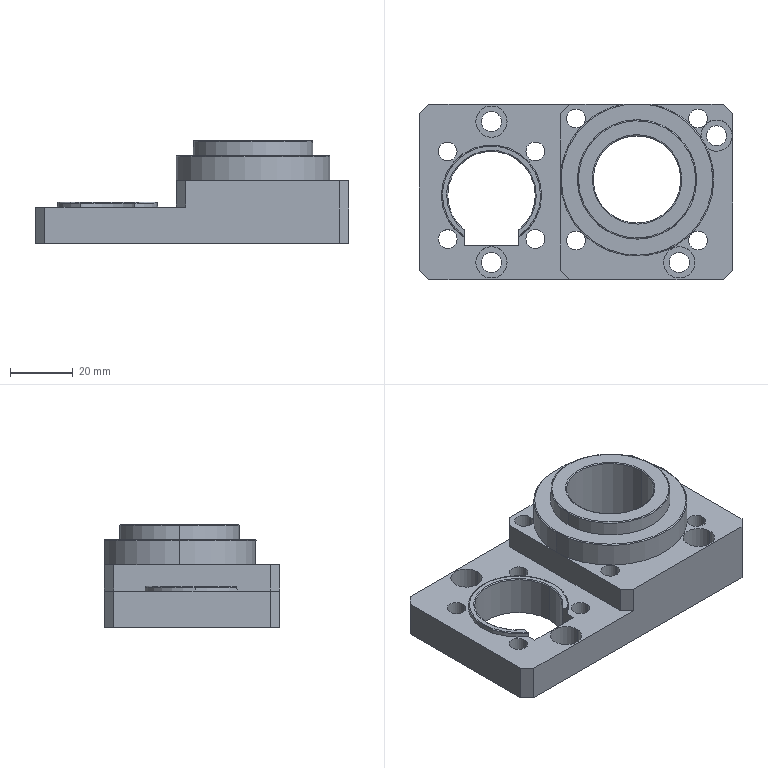Part | SolidWorks | features BaseBody 1 | 1 solid | 84 faces | box 100 x 56 x 32.8 mm | volume 75524 mm3 | cylinder 40 | plane 26 | spline 13 | cone 5 | commonest cylinder face diameters 6 x16 6.4 x8 10 x8 28 x5 49 x3